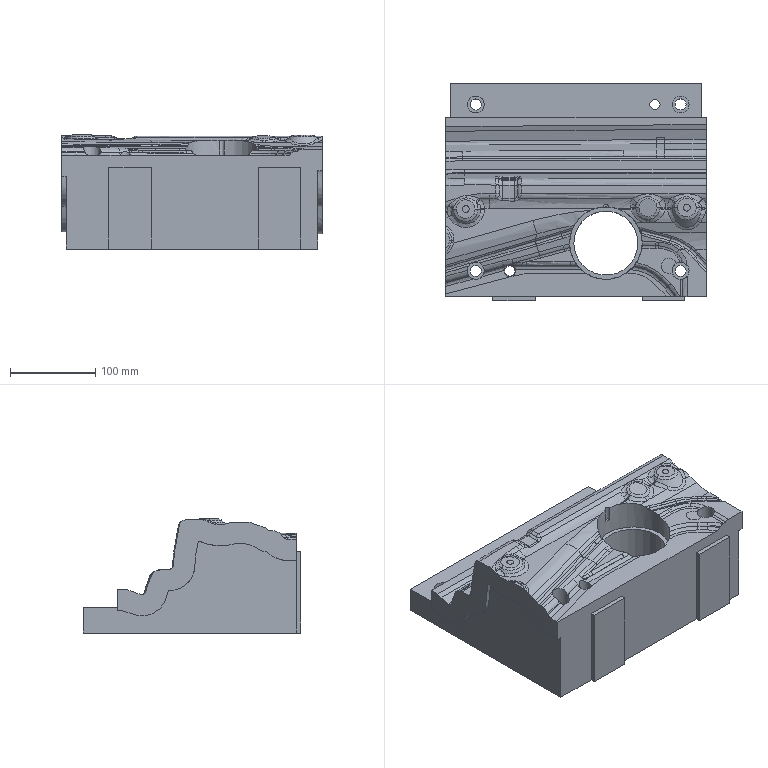Part | NX | features solid 2 | 1 solid | 293 faces | box 305.811 x 255 x 133.61 mm | volume 6122211 mm3 | spline 255 | plane 24 | cylinder 14 | commonest cylinder face diameters 13 x4 20 x4 12 x2 6 x1 14 x1 75 x1